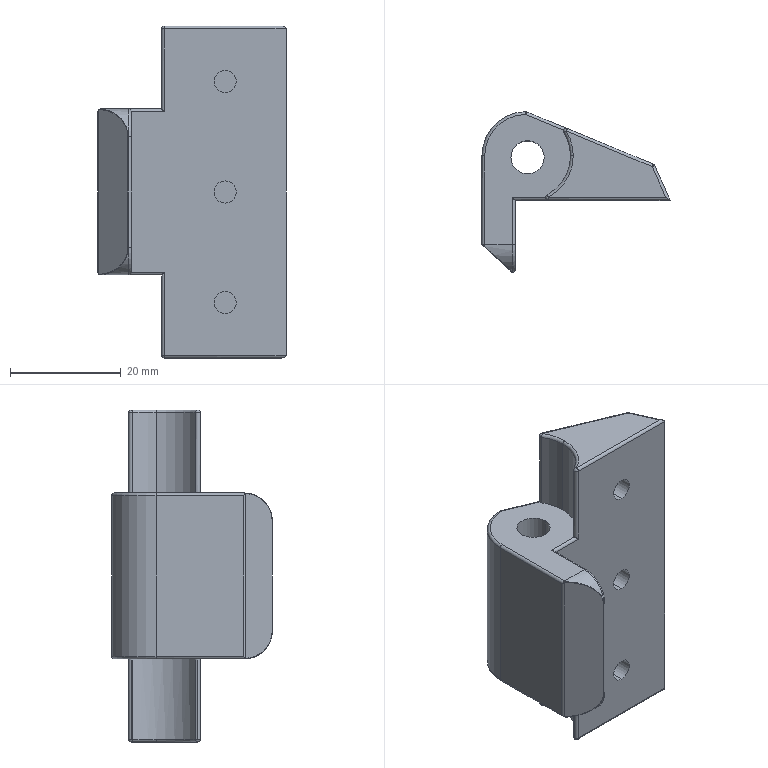Part | STEP file | Hinge movable plate | 1 solid | 79 faces | box 34 x 28.999 x 60 mm | volume 17414 mm3 | cylinder 39 | plane 14 | torus 10 | spline 8 | sphere 8 | commonest cylinder face diameters 1 x24 4 x6 16 x4 6 x2 10 x2 0.2 x1